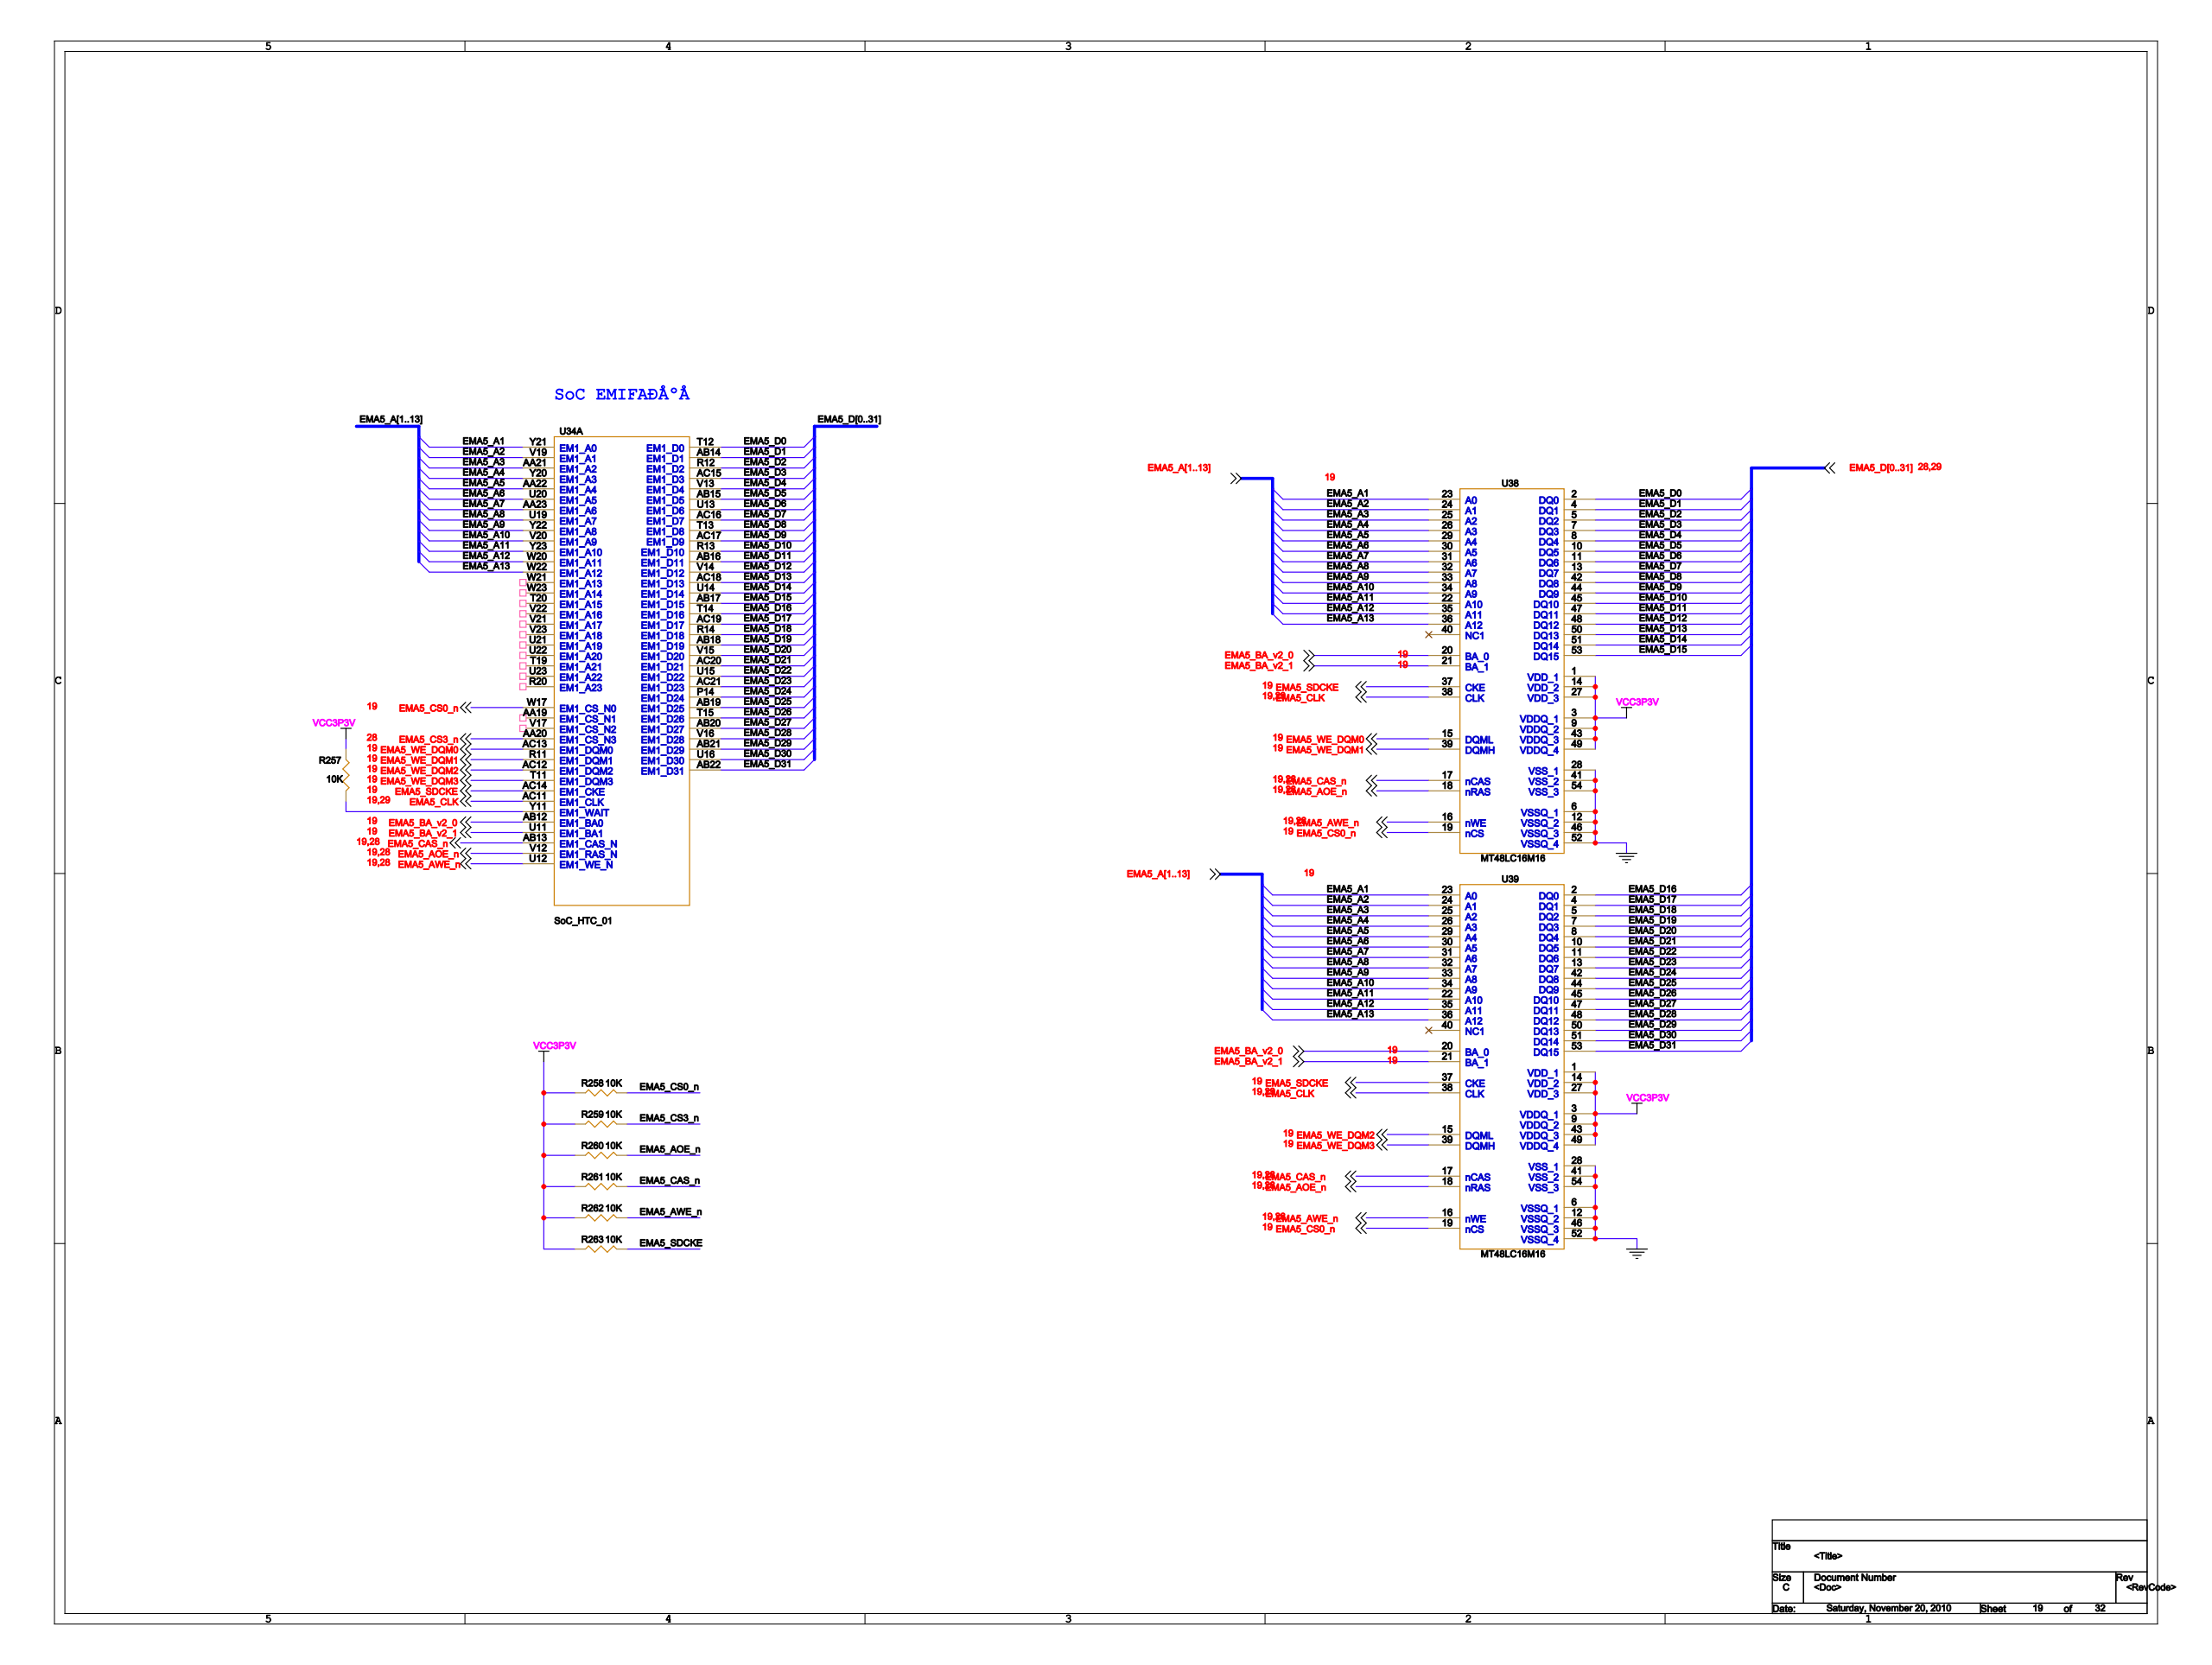Circuit board | Cadence Allegro | 1001 parts | 1318 nets | one sheet of the schematic
Parts on this sheet (reference | value | footprint):
R257 | 10K | 0603
R258 | 10K | 0603
R259 | 10K | 0603
R260 | 10K | 0603
R261 | 10K | 0603
R262 | 10K | 0603
R263 | 10K | 0603
U11 | MT48LC32M16 | TSOP54
U14 | MT48LC16M16 | TSOP54
U15 | MT48LC16M16 | TSOP54
U20 | MT48LC16M16 | TSOP54
U21 | MT48LC16M16 | TSOP54
U23 | MT48LC32M16 | TSOP54
U34 | SoC_HTC_01 | L529_XIN
U38 | MT48LC16M16 | TSOP54
U39 | MT48LC16M16 | TSOP54
Nets of these parts (net: part-pin ...):
EMA5_D20: U34-V15 U39-8
EMA5_D4: U34-V13 U38-8
EMA5_D12: U34-V14 U38-48
EMA5_CAS_N: R261-2 U34-AB13 U38-17 U39-17
EMA5_AOE_N: R260-2 U34-V12 U38-18 U39-18
EMA5_AWE_N: R262-2 U34-U12 U38-16 U39-16
EMA5_D0: U34-T12 U38-2
EMA5_D14: U34-U14 U38-51
EMA5_D2: U34-R12 U38-5
EMA5_CLK: U34-AC11 U38-38 U39-38
EMA5_D1: U34-AB14 U38-4
EMA5_D19: U34-AB18 U39-7
EMA5_D25: U34-AB19 U39-44
EMA5_D13: U34-AC18 U38-50
EMA5_D6: U34-U13 U38-11
EMA5_D30: U34-U16 U39-51
EMA5_D26: U34-T15 U39-45
EMA5_D18: U34-R14 U39-5
EMA5_D28: U34-V16 U39-48
EMA5_D8: U34-T13 U38-42
EMA5_D10: U34-R13 U38-45
EMA5_D16: U34-T14 U39-2
EMA5_D24: U34-P14 U39-42
EMA5_D22: U34-U15 U39-11
EMA5_CS3_N: R259-2 U34-AA20
EMA5_D31: U34-AB22 U39-53
EMA5_D29: U34-AB21 U39-50
EMA5_D23: U34-AC21 U39-13
EMA5_D5: U34-AB15 U38-10
EMA5_D3: U34-AC15 U38-7
EMA5_D11: U34-AB16 U38-47
EMA5_D7: U34-AC16 U38-13
EMA5_D15: U34-AB17 U38-53
EMA5_D9: U34-AC17 U38-44
EMA5_D17: U34-AC19 U39-4
EMA5_D27: U34-AB20 U39-47
EMA5_D21: U34-AC20 U39-10
VCC3P3V: R257-2 R258-1 R259-1 R260-1 R261-1 R262-1 R263-1 U11-1 U11-3 U11-9 U11-14 U11-27 U11-43 U11-49 U14-1 U14-3 U14-9 U14-14 U14-27 U14-43 U14-49 U15-1 U15-3 U15-9 U15-14 U15-27 U15-43 U15-49 U20-1 U20-3 U20-9 U20-14 U20-27 U20-43 U20-49 U21-1 U21-3 U21-9 U21-14 U21-27 U21-43 U21-49 U23-1 U23-3 U23-9 U23-14 U23-27 U23-43 U23-49 U38-1 U38-3 U38-9 U38-14 U38-27 U38-43 U38-49 U39-1 U39-3 U39-9 U39-14 U39-27 U39-43 U39-49
EMA5_A1: U34-Y21 U38-23 U39-23
EMA5_A2: U34-V19 U38-24 U39-24
EMA5_A11: U34-Y23 U38-22 U39-22
EMA5_A12: U34-W20 U38-35 U39-35
EMA5_A13: U34-W22 U38-36 U39-36
EMA5_A3: U34-AA21 U38-25 U39-25
EMA5_A4: U34-Y20 U38-26 U39-26
EMA5_A5: U34-AA22 U38-29 U39-29
EMA5_A6: U34-U20 U38-30 U39-30
EMA5_A7: U34-AA23 U38-31 U39-31
EMA5_A8: U34-U19 U38-32 U39-32
EMA5_A9: U34-Y22 U38-33 U39-33
EMA5_A10: U34-V20 U38-34 U39-34
EMA5_SDCKE: R263-2 U34-AC14 U38-37 U39-37
EMA5_CS0_N: R258-2 U34-W17 U38-19 U39-19
EMA5_WE_DQM0: U34-AC13 U38-15
EMA5_WE_DQM1: U34-R11 U38-39
EMA5_WE_DQM2: U34-AC12 U39-15
EMA5_WE_DQM3: U34-T11 U39-39
N16890328: R257-1 U34-Y11